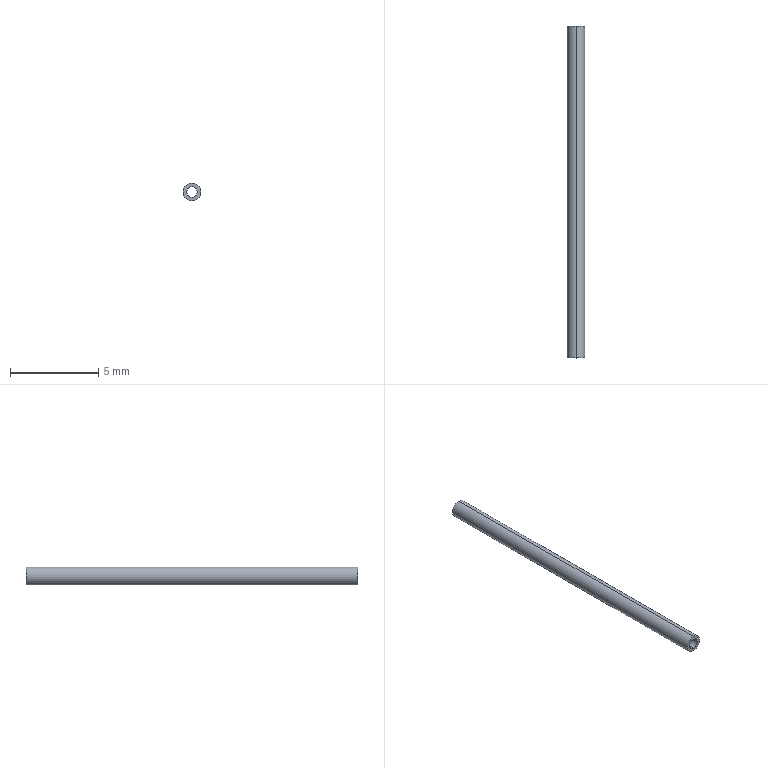Part | SolidWorks | features Revolution 1 | 1 solid | 6 faces | box 1 x 18.84 x 1 mm | volume 9.47 mm3 | cylinder 4 | plane 2 | commonest cylinder face diameters 0.6 x2 1 x2
STEP:
#1=CARTESIAN_POINT('',(0.,0.,0.5));
#2=VERTEX_POINT('',#1);
#3=CARTESIAN_POINT('',(0.,0.,-0.5));
#4=VERTEX_POINT('',#3);
#5=CARTESIAN_POINT('',(0.,0.,0.));
#6=DIRECTION('',(0.,1.,0.));
#7=DIRECTION('',(0.,0.,1.));
#8=AXIS2_PLACEMENT_3D('',#5,#6,#7);
#9=CIRCLE('',#8,0.5);
#10=EDGE_CURVE('',#2,#4,#9,.T.);
#11=ORIENTED_EDGE('',*,*,#10,.T.);
#12=CARTESIAN_POINT('',(0.,18.84,-0.5));
#13=VERTEX_POINT('',#12);
#14=CARTESIAN_POINT('',(0.,23.646,-0.5));
#15=DIRECTION('',(0.,1.,0.));
#16=VECTOR('',#15,1000.);
#17=LINE('',#14,#16);
#18=EDGE_CURVE('',#4,#13,#17,.T.);
#19=ORIENTED_EDGE('',*,*,#18,.T.);
#20=CARTESIAN_POINT('',(0.,18.84,0.5));
#21=VERTEX_POINT('',#20);
#22=CARTESIAN_POINT('',(0.,18.84,0.));
#23=DIRECTION('',(0.,1.,0.));
#24=DIRECTION('',(0.,0.,1.));
#25=AXIS2_PLACEMENT_3D('',#22,#23,#24);
#26=CIRCLE('',#25,0.5);
#27=EDGE_CURVE('',#21,#13,#26,.T.);
#28=ORIENTED_EDGE('',*,*,#27,.F.);
#29=CARTESIAN_POINT('',(0.,23.646,0.5));
#30=DIRECTION('',(0.,1.,0.));
#31=VECTOR('',#30,1000.);
#32=LINE('',#29,#31);
#33=EDGE_CURVE('',#2,#21,#32,.T.);
#34=ORIENTED_EDGE('',*,*,#33,.F.);
#35=EDGE_LOOP('',(#11,#19,#28,#34));
#36=FACE_OUTER_BOUND('',#35,.T.);
#37=CARTESIAN_POINT('',(0.,23.646,0.));
#38=DIRECTION('',(0.,1.,0.));
#39=DIRECTION('',(0.,0.,1.));
#40=AXIS2_PLACEMENT_3D('',#37,#38,#39);
#41=CYLINDRICAL_SURFACE('',#40,0.5);
#42=ADVANCED_FACE('',(#36),#41,.T.);
#43=CARTESIAN_POINT('',(0.,0.,-0.3));
#44=VERTEX_POINT('',#43);
#45=CARTESIAN_POINT('',(0.,0.,0.3));
#46=VERTEX_POINT('',#45);
#47=CARTESIAN_POINT('',(0.,0.,0.));
#48=DIRECTION('',(0.,1.,0.));
#49=DIRECTION('',(0.,0.,1.));
#50=AXIS2_PLACEMENT_3D('',#47,#48,#49);
#51=CIRCLE('',#50,0.3);
#52=EDGE_CURVE('',#44,#46,#51,.T.);
#53=ORIENTED_EDGE('',*,*,#52,.F.);
#54=CARTESIAN_POINT('',(0.,18.84,-0.3));
#55=VERTEX_POINT('',#54);
#56=CARTESIAN_POINT('',(0.,23.646,-0.3));
#57=DIRECTION('',(0.,1.,0.));
#58=VECTOR('',#57,1000.);
#59=LINE('',#56,#58);
#60=EDGE_CURVE('',#44,#55,#59,.T.);
#61=ORIENTED_EDGE('',*,*,#60,.T.);
#62=CARTESIAN_POINT('',(0.,18.84,0.3));
#63=VERTEX_POINT('',#62);
#64=CARTESIAN_POINT('',(0.,18.84,0.));
#65=DIRECTION('',(0.,1.,0.));
#66=DIRECTION('',(0.,0.,1.));
#67=AXIS2_PLACEMENT_3D('',#64,#65,#66);
#68=CIRCLE('',#67,0.3);
#69=EDGE_CURVE('',#55,#63,#68,.T.);
#70=ORIENTED_EDGE('',*,*,#69,.T.);
#71=CARTESIAN_POINT('',(0.,23.646,0.3));
#72=DIRECTION('',(0.,1.,0.));
#73=VECTOR('',#72,1000.);
#74=LINE('',#71,#73);
#75=EDGE_CURVE('',#46,#63,#74,.T.);
#76=ORIENTED_EDGE('',*,*,#75,.F.);
#77=EDGE_LOOP('',(#53,#61,#70,#76));
#78=FACE_OUTER_BOUND('',#77,.T.);
#79=CARTESIAN_POINT('',(0.,23.646,0.));
#80=DIRECTION('',(0.,1.,0.));
#81=DIRECTION('',(0.,0.,1.));
#82=AXIS2_PLACEMENT_3D('',#79,#80,#81);
#83=CYLINDRICAL_SURFACE('',#82,0.3);
#84=ADVANCED_FACE('',(#78),#83,.F.);
#85=ORIENTED_EDGE('',*,*,#27,.T.);
#86=CARTESIAN_POINT('',(0.,18.84,0.));
#87=DIRECTION('',(0.,1.,0.));
#88=DIRECTION('',(0.,0.,1.));
#89=AXIS2_PLACEMENT_3D('',#86,#87,#88);
#90=CIRCLE('',#89,0.5);
#91=EDGE_CURVE('',#13,#21,#90,.T.);
#92=ORIENTED_EDGE('',*,*,#91,.T.);
#93=EDGE_LOOP('',(#85,#92));
#94=FACE_OUTER_BOUND('',#93,.T.);
#95=CARTESIAN_POINT('',(0.,18.84,0.));
#96=DIRECTION('',(0.,1.,0.));
#97=DIRECTION('',(0.,0.,1.));
#98=AXIS2_PLACEMENT_3D('',#95,#96,#97);
#99=CIRCLE('',#98,0.3);
#100=EDGE_CURVE('',#63,#55,#99,.T.);
#101=ORIENTED_EDGE('',*,*,#100,.F.);
#102=ORIENTED_EDGE('',*,*,#69,.F.);
#103=EDGE_LOOP('',(#101,#102));
#104=FACE_BOUND('',#103,.T.);
#105=CARTESIAN_POINT('',(-0.5,18.84,0.));
#106=DIRECTION('',(0.,1.,0.));
#107=DIRECTION('',(0.,0.,1.));
#108=AXIS2_PLACEMENT_3D('',#105,#106,#107);
#109=PLANE('',#108);
#110=ADVANCED_FACE('',(#94,#104),#109,.T.);
#111=ORIENTED_EDGE('',*,*,#60,.F.);
#112=CARTESIAN_POINT('',(0.,0.,0.));
#113=DIRECTION('',(0.,1.,0.));
#114=DIRECTION('',(0.,0.,1.));
#115=AXIS2_PLACEMENT_3D('',#112,#113,#114);
#116=CIRCLE('',#115,0.3);
#117=EDGE_CURVE('',#46,#44,#116,.T.);
#118=ORIENTED_EDGE('',*,*,#117,.F.);
#119=ORIENTED_EDGE('',*,*,#75,.T.);
#120=ORIENTED_EDGE('',*,*,#100,.T.);
#121=EDGE_LOOP('',(#111,#118,#119,#120));
#122=FACE_OUTER_BOUND('',#121,.T.);
#123=CARTESIAN_POINT('',(0.,23.646,0.));
#124=DIRECTION('',(0.,1.,0.));
#125=DIRECTION('',(0.,0.,1.));
#126=AXIS2_PLACEMENT_3D('',#123,#124,#125);
#127=CYLINDRICAL_SURFACE('',#126,0.3);
#128=ADVANCED_FACE('',(#122),#127,.F.);
#129=ORIENTED_EDGE('',*,*,#117,.T.);
#130=ORIENTED_EDGE('',*,*,#52,.T.);
#131=EDGE_LOOP('',(#129,#130));
#132=FACE_BOUND('',#131,.T.);
#133=ORIENTED_EDGE('',*,*,#10,.F.);
#134=CARTESIAN_POINT('',(0.,0.,0.));
#135=DIRECTION('',(0.,1.,0.));
#136=DIRECTION('',(0.,0.,1.));
#137=AXIS2_PLACEMENT_3D('',#134,#135,#136);
#138=CIRCLE('',#137,0.5);
#139=EDGE_CURVE('',#4,#2,#138,.T.);
#140=ORIENTED_EDGE('',*,*,#139,.F.);
#141=EDGE_LOOP('',(#133,#140));
#142=FACE_OUTER_BOUND('',#141,.T.);
#143=CARTESIAN_POINT('',(-0.5,0.,0.));
#144=DIRECTION('',(0.,-1.,0.));
#145=DIRECTION('',(0.,0.,-1.));
#146=AXIS2_PLACEMENT_3D('',#143,#144,#145);
#147=PLANE('',#146);
#148=ADVANCED_FACE('',(#132,#142),#147,.T.);
#149=ORIENTED_EDGE('',*,*,#18,.F.);
#150=ORIENTED_EDGE('',*,*,#139,.T.);
#151=ORIENTED_EDGE('',*,*,#33,.T.);
#152=ORIENTED_EDGE('',*,*,#91,.F.);
#153=EDGE_LOOP('',(#149,#150,#151,#152));
#154=FACE_OUTER_BOUND('',#153,.T.);
#155=CARTESIAN_POINT('',(0.,23.646,0.));
#156=DIRECTION('',(0.,1.,0.));
#157=DIRECTION('',(0.,0.,1.));
#158=AXIS2_PLACEMENT_3D('',#155,#156,#157);
#159=CYLINDRICAL_SURFACE('',#158,0.5);
#160=ADVANCED_FACE('',(#154),#159,.T.);
#161=CLOSED_SHELL('',(#42,#84,#110,#128,#148,#160));
#162=MANIFOLD_SOLID_BREP('',#161);
#163=CARTESIAN_POINT('',(0.,0.,0.));
#164=DIRECTION('',(0.,0.,1.));
#165=DIRECTION('',(1.,0.,0.));
#166=AXIS2_PLACEMENT_3D('',#163,#164,#165);
#167=(LENGTH_UNIT()NAMED_UNIT(*)SI_UNIT(.MILLI.,.METRE.));
#168=UNCERTAINTY_MEASURE_WITH_UNIT(LENGTH_MEASURE(0.00001),#167,'','');
#169=(NAMED_UNIT(*)PLANE_ANGLE_UNIT()SI_UNIT($,.RADIAN.));
#170=(NAMED_UNIT(*)SI_UNIT($,.STERADIAN.)SOLID_ANGLE_UNIT());
#171=(GEOMETRIC_REPRESENTATION_CONTEXT(3)GLOBAL_UNCERTAINTY_ASSIGNED_CONTEXT((#168))GLOBAL_UNIT_ASSIGNED_CONTEXT((#167,#169,#170))REPRESENTATION_CONTEXT('',''));
#172=ADVANCED_BREP_SHAPE_REPRESENTATION('',(#162,#166),#171);